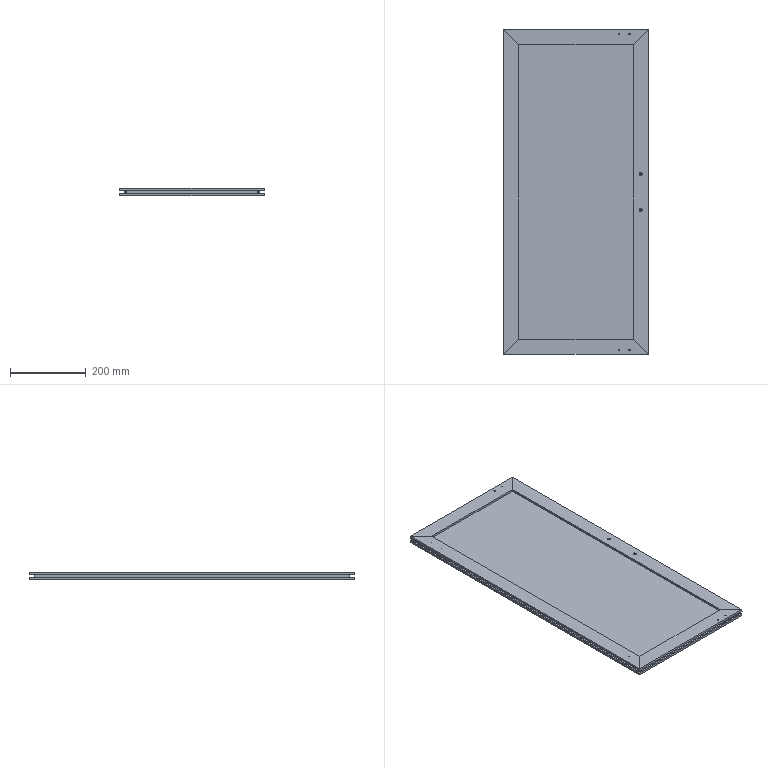Part | SolidWorks | features HoleWzd 3, ICE 1, WeldMemberFeat 1, WeldmentFeature 1 | 5 solids | 184 faces | box 382 x 856 x 20 mm | volume 2117530 mm3 | plane 132 | cylinder 44 | cone 8 | commonest cylinder face diameters 5 x16 3.3 x8 4.5 x8 6.5 x8 8 x4